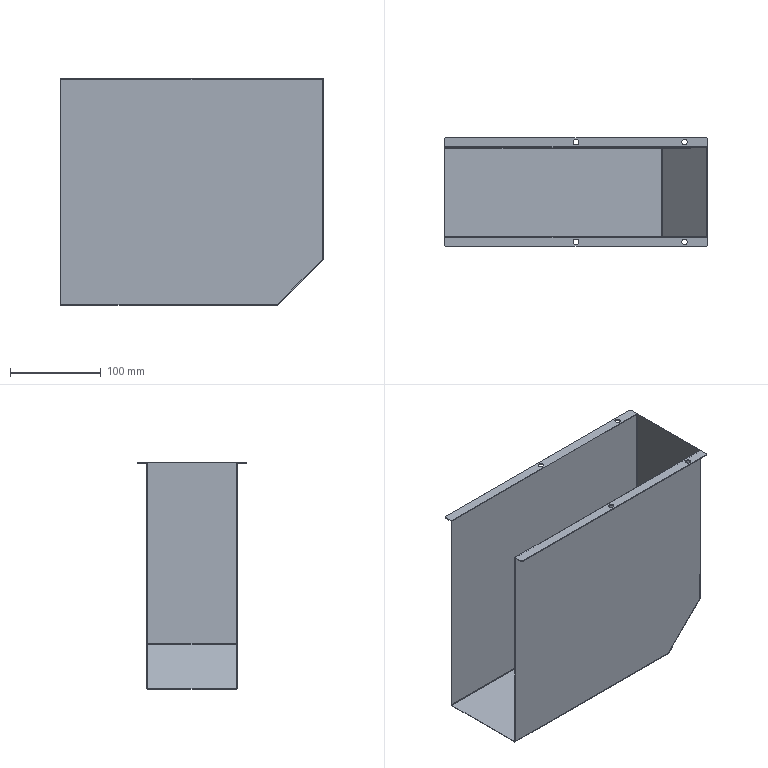Part | NX | features BREP 1 | 1 solid | 54 faces | box 290 x 120 x 250 mm | volume 102028 mm3 | cylinder 28 | plane 18 | sphere 8 | commonest cylinder face diameters 2 x12 1 x8 6 x8
STEP:
#1=CARTESIAN_POINT('',(-3.,55.,250.));
#2=VERTEX_POINT('',#1);
#3=CARTESIAN_POINT('',(3.,55.,250.));
#4=VERTEX_POINT('',#3);
#5=CARTESIAN_POINT('',(0.,55.,250.));
#6=DIRECTION('',(0.,0.,1.));
#7=DIRECTION('',(-1.,0.,0.));
#8=AXIS2_PLACEMENT_3D('',#5,#6,#7);
#9=CIRCLE('',#8,3.);
#10=EDGE_CURVE('',#2,#4,#9,.T.);
#11=ORIENTED_EDGE('',*,*,#10,.T.);
#12=CARTESIAN_POINT('',(3.,55.,249.));
#13=VERTEX_POINT('',#12);
#14=CARTESIAN_POINT('',(3.,55.,250.));
#15=DIRECTION('',(0.,0.,-1.));
#16=VECTOR('',#15,1000.);
#17=LINE('',#14,#16);
#18=EDGE_CURVE('',#4,#13,#17,.T.);
#19=ORIENTED_EDGE('',*,*,#18,.T.);
#20=CARTESIAN_POINT('',(-3.,55.,249.));
#21=VERTEX_POINT('',#20);
#22=CARTESIAN_POINT('',(0.,55.,249.));
#23=DIRECTION('',(0.,0.,1.));
#24=DIRECTION('',(-1.,0.,0.));
#25=AXIS2_PLACEMENT_3D('',#22,#23,#24);
#26=CIRCLE('',#25,3.);
#27=EDGE_CURVE('',#21,#13,#26,.T.);
#28=ORIENTED_EDGE('',*,*,#27,.F.);
#29=CARTESIAN_POINT('',(-3.,55.,250.));
#30=DIRECTION('',(0.,0.,-1.));
#31=VECTOR('',#30,1000.);
#32=LINE('',#29,#31);
#33=EDGE_CURVE('',#2,#21,#32,.T.);
#34=ORIENTED_EDGE('',*,*,#33,.F.);
#35=EDGE_LOOP('',(#11,#19,#28,#34));
#36=FACE_BOUND('',#35,.T.);
#37=CARTESIAN_POINT('',(0.,55.,250.));
#38=DIRECTION('',(0.,0.,-1.));
#39=DIRECTION('',(-1.,0.,0.));
#40=AXIS2_PLACEMENT_3D('',#37,#38,#39);
#41=CYLINDRICAL_SURFACE('',#40,3.);
#42=ADVANCED_FACE('',(#36),#41,.F.);
#43=CARTESIAN_POINT('',(117.,55.,250.));
#44=VERTEX_POINT('',#43);
#45=CARTESIAN_POINT('',(123.,55.,250.));
#46=VERTEX_POINT('',#45);
#47=CARTESIAN_POINT('',(120.,55.,250.));
#48=DIRECTION('',(0.,0.,1.));
#49=DIRECTION('',(-1.,0.,0.));
#50=AXIS2_PLACEMENT_3D('',#47,#48,#49);
#51=CIRCLE('',#50,3.);
#52=EDGE_CURVE('',#44,#46,#51,.T.);
#53=ORIENTED_EDGE('',*,*,#52,.T.);
#54=CARTESIAN_POINT('',(123.,55.,249.));
#55=VERTEX_POINT('',#54);
#56=CARTESIAN_POINT('',(123.,55.,250.));
#57=DIRECTION('',(0.,0.,-1.));
#58=VECTOR('',#57,1000.);
#59=LINE('',#56,#58);
#60=EDGE_CURVE('',#46,#55,#59,.T.);
#61=ORIENTED_EDGE('',*,*,#60,.T.);
#62=CARTESIAN_POINT('',(117.,55.,249.));
#63=VERTEX_POINT('',#62);
#64=CARTESIAN_POINT('',(120.,55.,249.));
#65=DIRECTION('',(0.,0.,1.));
#66=DIRECTION('',(-1.,0.,0.));
#67=AXIS2_PLACEMENT_3D('',#64,#65,#66);
#68=CIRCLE('',#67,3.);
#69=EDGE_CURVE('',#63,#55,#68,.T.);
#70=ORIENTED_EDGE('',*,*,#69,.F.);
#71=CARTESIAN_POINT('',(117.,55.,250.));
#72=DIRECTION('',(0.,0.,-1.));
#73=VECTOR('',#72,1000.);
#74=LINE('',#71,#73);
#75=EDGE_CURVE('',#44,#63,#74,.T.);
#76=ORIENTED_EDGE('',*,*,#75,.F.);
#77=EDGE_LOOP('',(#53,#61,#70,#76));
#78=FACE_BOUND('',#77,.T.);
#79=CARTESIAN_POINT('',(120.,55.,250.));
#80=DIRECTION('',(0.,0.,-1.));
#81=DIRECTION('',(-1.,0.,0.));
#82=AXIS2_PLACEMENT_3D('',#79,#80,#81);
#83=CYLINDRICAL_SURFACE('',#82,3.);
#84=ADVANCED_FACE('',(#78),#83,.F.);
#85=CARTESIAN_POINT('',(3.,-55.,250.));
#86=VERTEX_POINT('',#85);
#87=CARTESIAN_POINT('',(-3.,-55.,250.));
#88=VERTEX_POINT('',#87);
#89=CARTESIAN_POINT('',(0.,-55.,250.));
#90=DIRECTION('',(0.,0.,-1.));
#91=DIRECTION('',(-1.,0.,0.));
#92=AXIS2_PLACEMENT_3D('',#89,#90,#91);
#93=CIRCLE('',#92,3.);
#94=EDGE_CURVE('',#86,#88,#93,.T.);
#95=ORIENTED_EDGE('',*,*,#94,.F.);
#96=CARTESIAN_POINT('',(3.,-55.,249.));
#97=VERTEX_POINT('',#96);
#98=CARTESIAN_POINT('',(3.,-55.,250.));
#99=DIRECTION('',(0.,0.,-1.));
#100=VECTOR('',#99,1000.);
#101=LINE('',#98,#100);
#102=EDGE_CURVE('',#86,#97,#101,.T.);
#103=ORIENTED_EDGE('',*,*,#102,.T.);
#104=CARTESIAN_POINT('',(-3.,-55.,249.));
#105=VERTEX_POINT('',#104);
#106=CARTESIAN_POINT('',(0.,-55.,249.));
#107=DIRECTION('',(0.,0.,-1.));
#108=DIRECTION('',(-1.,0.,0.));
#109=AXIS2_PLACEMENT_3D('',#106,#107,#108);
#110=CIRCLE('',#109,3.);
#111=EDGE_CURVE('',#97,#105,#110,.T.);
#112=ORIENTED_EDGE('',*,*,#111,.T.);
#113=CARTESIAN_POINT('',(-3.,-55.,250.));
#114=DIRECTION('',(0.,0.,-1.));
#115=VECTOR('',#114,1000.);
#116=LINE('',#113,#115);
#117=EDGE_CURVE('',#88,#105,#116,.T.);
#118=ORIENTED_EDGE('',*,*,#117,.F.);
#119=EDGE_LOOP('',(#95,#103,#112,#118));
#120=FACE_BOUND('',#119,.T.);
#121=CARTESIAN_POINT('',(0.,-55.,250.));
#122=DIRECTION('',(0.,0.,-1.));
#123=DIRECTION('',(-1.,0.,0.));
#124=AXIS2_PLACEMENT_3D('',#121,#122,#123);
#125=CYLINDRICAL_SURFACE('',#124,3.);
#126=ADVANCED_FACE('',(#120),#125,.F.);
#127=CARTESIAN_POINT('',(123.,-55.,250.));
#128=VERTEX_POINT('',#127);
#129=CARTESIAN_POINT('',(117.,-55.,250.));
#130=VERTEX_POINT('',#129);
#131=CARTESIAN_POINT('',(120.,-55.,250.));
#132=DIRECTION('',(0.,0.,-1.));
#133=DIRECTION('',(-1.,0.,0.));
#134=AXIS2_PLACEMENT_3D('',#131,#132,#133);
#135=CIRCLE('',#134,3.);
#136=EDGE_CURVE('',#128,#130,#135,.T.);
#137=ORIENTED_EDGE('',*,*,#136,.F.);
#138=CARTESIAN_POINT('',(123.,-55.,249.));
#139=VERTEX_POINT('',#138);
#140=CARTESIAN_POINT('',(123.,-55.,250.));
#141=DIRECTION('',(0.,0.,-1.));
#142=VECTOR('',#141,1000.);
#143=LINE('',#140,#142);
#144=EDGE_CURVE('',#128,#139,#143,.T.);
#145=ORIENTED_EDGE('',*,*,#144,.T.);
#146=CARTESIAN_POINT('',(117.,-55.,249.));
#147=VERTEX_POINT('',#146);
#148=CARTESIAN_POINT('',(120.,-55.,249.));
#149=DIRECTION('',(0.,0.,-1.));
#150=DIRECTION('',(-1.,0.,0.));
#151=AXIS2_PLACEMENT_3D('',#148,#149,#150);
#152=CIRCLE('',#151,3.);
#153=EDGE_CURVE('',#139,#147,#152,.T.);
#154=ORIENTED_EDGE('',*,*,#153,.T.);
#155=CARTESIAN_POINT('',(117.,-55.,250.));
#156=DIRECTION('',(0.,0.,-1.));
#157=VECTOR('',#156,1000.);
#158=LINE('',#155,#157);
#159=EDGE_CURVE('',#130,#147,#158,.T.);
#160=ORIENTED_EDGE('',*,*,#159,.F.);
#161=EDGE_LOOP('',(#137,#145,#154,#160));
#162=FACE_BOUND('',#161,.T.);
#163=CARTESIAN_POINT('',(120.,-55.,250.));
#164=DIRECTION('',(0.,0.,-1.));
#165=DIRECTION('',(-1.,0.,0.));
#166=AXIS2_PLACEMENT_3D('',#163,#164,#165);
#167=CYLINDRICAL_SURFACE('',#166,3.);
#168=ADVANCED_FACE('',(#162),#167,.F.);
#169=CARTESIAN_POINT('',(144.,60.,250.));
#170=VERTEX_POINT('',#169);
#171=CARTESIAN_POINT('',(-144.,60.,250.));
#172=VERTEX_POINT('',#171);
#173=CARTESIAN_POINT('',(145.,60.,250.));
#174=DIRECTION('',(-1.,0.,0.));
#175=VECTOR('',#174,1000.);
#176=LINE('',#173,#175);
#177=EDGE_CURVE('',#170,#172,#176,.T.);
#178=ORIENTED_EDGE('',*,*,#177,.T.);
#179=CARTESIAN_POINT('',(-145.,59.,250.));
#180=VERTEX_POINT('',#179);
#181=CARTESIAN_POINT('',(-144.,59.,250.));
#182=DIRECTION('',(0.,0.,1.));
#183=DIRECTION('',(-1.,0.,0.));
#184=AXIS2_PLACEMENT_3D('',#181,#182,#183);
#185=CIRCLE('',#184,1.);
#186=EDGE_CURVE('',#172,#180,#185,.T.);
#187=ORIENTED_EDGE('',*,*,#186,.T.);
#188=CARTESIAN_POINT('',(-145.,49.5,250.));
#189=VERTEX_POINT('',#188);
#190=CARTESIAN_POINT('',(-145.,-50.,250.));
#191=DIRECTION('',(0.,-1.,0.));
#192=VECTOR('',#191,1000.);
#193=LINE('',#190,#192);
#194=EDGE_CURVE('',#180,#189,#193,.T.);
#195=ORIENTED_EDGE('',*,*,#194,.T.);
#196=CARTESIAN_POINT('',(144.,49.5,250.));
#197=VERTEX_POINT('',#196);
#198=CARTESIAN_POINT('',(0.,49.5,250.));
#199=DIRECTION('',(-1.,0.,0.));
#200=VECTOR('',#199,1000.);
#201=LINE('',#198,#200);
#202=EDGE_CURVE('',#197,#189,#201,.T.);
#203=ORIENTED_EDGE('',*,*,#202,.F.);
#204=CARTESIAN_POINT('',(144.5,49.,250.));
#205=VERTEX_POINT('',#204);
#206=CARTESIAN_POINT('',(144.,49.,250.));
#207=DIRECTION('',(0.,0.,-1.));
#208=DIRECTION('',(-1.,0.,0.));
#209=AXIS2_PLACEMENT_3D('',#206,#207,#208);
#210=CIRCLE('',#209,0.5);
#211=EDGE_CURVE('',#197,#205,#210,.T.);
#212=ORIENTED_EDGE('',*,*,#211,.T.);
#213=CARTESIAN_POINT('',(144.5,-49.,250.));
#214=VERTEX_POINT('',#213);
#215=CARTESIAN_POINT('',(144.5,0.,250.));
#216=DIRECTION('',(0.,1.,0.));
#217=VECTOR('',#216,1000.);
#218=LINE('',#215,#217);
#219=EDGE_CURVE('',#214,#205,#218,.T.);
#220=ORIENTED_EDGE('',*,*,#219,.F.);
#221=CARTESIAN_POINT('',(144.,-49.5,250.));
#222=VERTEX_POINT('',#221);
#223=CARTESIAN_POINT('',(144.,-49.,250.));
#224=DIRECTION('',(0.,0.,-1.));
#225=DIRECTION('',(-1.,0.,0.));
#226=AXIS2_PLACEMENT_3D('',#223,#224,#225);
#227=CIRCLE('',#226,0.5);
#228=EDGE_CURVE('',#214,#222,#227,.T.);
#229=ORIENTED_EDGE('',*,*,#228,.T.);
#230=CARTESIAN_POINT('',(-145.,-49.5,250.));
#231=VERTEX_POINT('',#230);
#232=CARTESIAN_POINT('',(0.,-49.5,250.));
#233=DIRECTION('',(1.,0.,0.));
#234=VECTOR('',#233,1000.);
#235=LINE('',#232,#234);
#236=EDGE_CURVE('',#231,#222,#235,.T.);
#237=ORIENTED_EDGE('',*,*,#236,.F.);
#238=CARTESIAN_POINT('',(-145.,-59.,250.));
#239=VERTEX_POINT('',#238);
#240=CARTESIAN_POINT('',(-145.,-50.,250.));
#241=DIRECTION('',(0.,-1.,0.));
#242=VECTOR('',#241,1000.);
#243=LINE('',#240,#242);
#244=EDGE_CURVE('',#231,#239,#243,.T.);
#245=ORIENTED_EDGE('',*,*,#244,.T.);
#246=CARTESIAN_POINT('',(-144.,-60.,250.));
#247=VERTEX_POINT('',#246);
#248=CARTESIAN_POINT('',(-144.,-59.,250.));
#249=DIRECTION('',(0.,0.,1.));
#250=DIRECTION('',(-1.,0.,0.));
#251=AXIS2_PLACEMENT_3D('',#248,#249,#250);
#252=CIRCLE('',#251,1.);
#253=EDGE_CURVE('',#239,#247,#252,.T.);
#254=ORIENTED_EDGE('',*,*,#253,.T.);
#255=CARTESIAN_POINT('',(144.,-60.,250.));
#256=VERTEX_POINT('',#255);
#257=CARTESIAN_POINT('',(145.,-60.,250.));
#258=DIRECTION('',(-1.,0.,0.));
#259=VECTOR('',#258,1000.);
#260=LINE('',#257,#259);
#261=EDGE_CURVE('',#256,#247,#260,.T.);
#262=ORIENTED_EDGE('',*,*,#261,.F.);
#263=CARTESIAN_POINT('',(145.,-59.,250.));
#264=VERTEX_POINT('',#263);
#265=CARTESIAN_POINT('',(144.,-59.,250.));
#266=DIRECTION('',(0.,0.,1.));
#267=DIRECTION('',(-1.,0.,0.));
#268=AXIS2_PLACEMENT_3D('',#265,#266,#267);
#269=CIRCLE('',#268,1.);
#270=EDGE_CURVE('',#256,#264,#269,.T.);
#271=ORIENTED_EDGE('',*,*,#270,.T.);
#272=CARTESIAN_POINT('',(145.,49.,250.));
#273=VERTEX_POINT('',#272);
#274=CARTESIAN_POINT('',(145.,-50.,250.));
#275=DIRECTION('',(0.,1.,0.));
#276=VECTOR('',#275,1000.);
#277=LINE('',#274,#276);
#278=EDGE_CURVE('',#264,#273,#277,.T.);
#279=ORIENTED_EDGE('',*,*,#278,.T.);
#280=CARTESIAN_POINT('',(144.,50.,250.));
#281=VERTEX_POINT('',#280);
#282=CARTESIAN_POINT('',(144.,49.,250.));
#283=DIRECTION('',(0.,0.,1.));
#284=DIRECTION('',(-1.,0.,0.));
#285=AXIS2_PLACEMENT_3D('',#282,#283,#284);
#286=CIRCLE('',#285,1.);
#287=EDGE_CURVE('',#273,#281,#286,.T.);
#288=ORIENTED_EDGE('',*,*,#287,.T.);
#289=CARTESIAN_POINT('',(145.,50.,250.));
#290=VERTEX_POINT('',#289);
#291=CARTESIAN_POINT('',(145.,50.,250.));
#292=DIRECTION('',(-1.,0.,0.));
#293=VECTOR('',#292,1000.);
#294=LINE('',#291,#293);
#295=EDGE_CURVE('',#290,#281,#294,.T.);
#296=ORIENTED_EDGE('',*,*,#295,.F.);
#297=CARTESIAN_POINT('',(145.,59.,250.));
#298=VERTEX_POINT('',#297);
#299=CARTESIAN_POINT('',(145.,60.,250.));
#300=DIRECTION('',(0.,-1.,0.));
#301=VECTOR('',#300,1000.);
#302=LINE('',#299,#301);
#303=EDGE_CURVE('',#298,#290,#302,.T.);
#304=ORIENTED_EDGE('',*,*,#303,.F.);
#305=CARTESIAN_POINT('',(144.,59.,250.));
#306=DIRECTION('',(0.,0.,1.));
#307=DIRECTION('',(-1.,0.,0.));
#308=AXIS2_PLACEMENT_3D('',#305,#306,#307);
#309=CIRCLE('',#308,1.);
#310=EDGE_CURVE('',#298,#170,#309,.T.);
#311=ORIENTED_EDGE('',*,*,#310,.T.);
#312=EDGE_LOOP('',(#178,#187,#195,#203,#212,#220,#229,#237,#245,#254,#262,#271,#279,#288,#296,#304,#311));
#313=FACE_BOUND('',#312,.T.);
#314=ORIENTED_EDGE('',*,*,#52,.F.);
#315=CARTESIAN_POINT('',(120.,55.,250.));
#316=DIRECTION('',(0.,0.,1.));
#317=DIRECTION('',(-1.,0.,0.));
#318=AXIS2_PLACEMENT_3D('',#315,#316,#317);
#319=CIRCLE('',#318,3.);
#320=EDGE_CURVE('',#46,#44,#319,.T.);
#321=ORIENTED_EDGE('',*,*,#320,.F.);
#322=EDGE_LOOP('',(#314,#321));
#323=FACE_BOUND('',#322,.T.);
#324=CARTESIAN_POINT('',(0.,-55.,250.));
#325=DIRECTION('',(0.,0.,-1.));
#326=DIRECTION('',(-1.,0.,0.));
#327=AXIS2_PLACEMENT_3D('',#324,#325,#326);
#328=CIRCLE('',#327,3.);
#329=EDGE_CURVE('',#88,#86,#328,.T.);
#330=ORIENTED_EDGE('',*,*,#329,.T.);
#331=ORIENTED_EDGE('',*,*,#94,.T.);
#332=EDGE_LOOP('',(#330,#331));
#333=FACE_BOUND('',#332,.T.);
#334=CARTESIAN_POINT('',(120.,-55.,250.));
#335=DIRECTION('',(0.,0.,-1.));
#336=DIRECTION('',(-1.,0.,0.));
#337=AXIS2_PLACEMENT_3D('',#334,#335,#336);
#338=CIRCLE('',#337,3.);
#339=EDGE_CURVE('',#130,#128,#338,.T.);
#340=ORIENTED_EDGE('',*,*,#339,.T.);
#341=ORIENTED_EDGE('',*,*,#136,.T.);
#342=EDGE_LOOP('',(#340,#341));
#343=FACE_BOUND('',#342,.T.);
#344=ORIENTED_EDGE('',*,*,#10,.F.);
#345=CARTESIAN_POINT('',(0.,55.,250.));
#346=DIRECTION('',(0.,0.,1.));
#347=DIRECTION('',(-1.,0.,0.));
#348=AXIS2_PLACEMENT_3D('',#345,#346,#347);
#349=CIRCLE('',#348,3.);
#350=EDGE_CURVE('',#4,#2,#349,.T.);
#351=ORIENTED_EDGE('',*,*,#350,.F.);
#352=EDGE_LOOP('',(#344,#351));
#353=FACE_BOUND('',#352,.T.);
#354=CARTESIAN_POINT('',(0.,0.,250.));
#355=DIRECTION('',(0.,0.,-1.));
#356=DIRECTION('',(0.,-1.,0.));
#357=AXIS2_PLACEMENT_3D('',#354,#355,#356);
#358=PLANE('',#357);
#359=ADVANCED_FACE('',(#313,#323,#333,#343,#353),#358,.F.);
#360=CARTESIAN_POINT('',(-145.,59.,249.));
#361=VERTEX_POINT('',#360);
#362=CARTESIAN_POINT('',(-145.,50.,249.));
#363=VERTEX_POINT('',#362);
#364=CARTESIAN_POINT('',(-145.,60.,249.));
#365=DIRECTION('',(0.,-1.,0.));
#366=VECTOR('',#365,1000.);
#367=LINE('',#364,#366);
#368=EDGE_CURVE('',#361,#363,#367,.T.);
#369=ORIENTED_EDGE('',*,*,#368,.F.);
#370=CARTESIAN_POINT('',(-144.,60.,249.));
#371=VERTEX_POINT('',#370);
#372=CARTESIAN_POINT('',(-144.,59.,249.));
#373=DIRECTION('',(0.,0.,-1.));
#374=DIRECTION('',(-1.,0.,0.));
#375=AXIS2_PLACEMENT_3D('',#372,#373,#374);
#376=CIRCLE('',#375,1.);
#377=EDGE_CURVE('',#361,#371,#376,.T.);
#378=ORIENTED_EDGE('',*,*,#377,.T.);
#379=CARTESIAN_POINT('',(144.,60.,249.));
#380=VERTEX_POINT('',#379);
#381=CARTESIAN_POINT('',(145.,60.,249.));
#382=DIRECTION('',(1.,0.,0.));
#383=VECTOR('',#382,1000.);
#384=LINE('',#381,#383);
#385=EDGE_CURVE('',#371,#380,#384,.T.);
#386=ORIENTED_EDGE('',*,*,#385,.T.);
#387=CARTESIAN_POINT('',(145.,59.,249.));
#388=VERTEX_POINT('',#387);
#389=CARTESIAN_POINT('',(144.,59.,249.));
#390=DIRECTION('',(0.,0.,-1.));
#391=DIRECTION('',(-1.,0.,0.));
#392=AXIS2_PLACEMENT_3D('',#389,#390,#391);
#393=CIRCLE('',#392,1.);
#394=EDGE_CURVE('',#380,#388,#393,.T.);
#395=ORIENTED_EDGE('',*,*,#394,.T.);
#396=CARTESIAN_POINT('',(145.,50.,249.));
#397=VERTEX_POINT('',#396);
#398=CARTESIAN_POINT('',(145.,60.,249.));
#399=DIRECTION('',(0.,-1.,0.));
#400=VECTOR('',#399,1000.);
#401=LINE('',#398,#400);
#402=EDGE_CURVE('',#388,#397,#401,.T.);
#403=ORIENTED_EDGE('',*,*,#402,.T.);
#404=CARTESIAN_POINT('',(144.,50.,249.));
#405=VERTEX_POINT('',#404);
#406=CARTESIAN_POINT('',(145.,50.,249.));
#407=DIRECTION('',(1.,0.,0.));
#408=VECTOR('',#407,1000.);
#409=LINE('',#406,#408);
#410=EDGE_CURVE('',#405,#397,#409,.T.);
#411=ORIENTED_EDGE('',*,*,#410,.F.);
#412=CARTESIAN_POINT('',(145.,50.,249.));
#413=DIRECTION('',(1.,0.,0.));
#414=VECTOR('',#413,1000.);
#415=LINE('',#412,#414);
#416=EDGE_CURVE('',#363,#405,#415,.T.);
#417=ORIENTED_EDGE('',*,*,#416,.F.);
#418=EDGE_LOOP('',(#369,#378,#386,#395,#403,#411,#417));
#419=FACE_BOUND('',#418,.T.);
#420=ORIENTED_EDGE('',*,*,#69,.T.);
#421=CARTESIAN_POINT('',(120.,55.,249.));
#422=DIRECTION('',(0.,0.,1.));
#423=DIRECTION('',(-1.,0.,0.));
#424=AXIS2_PLACEMENT_3D('',#421,#422,#423);
#425=CIRCLE('',#424,3.);
#426=EDGE_CURVE('',#55,#63,#425,.T.);
#427=ORIENTED_EDGE('',*,*,#426,.T.);
#428=EDGE_LOOP('',(#420,#427));
#429=FACE_BOUND('',#428,.T.);
#430=ORIENTED_EDGE('',*,*,#27,.T.);
#431=CARTESIAN_POINT('',(0.,55.,249.));
#432=DIRECTION('',(0.,0.,1.));
#433=DIRECTION('',(-1.,0.,0.));
#434=AXIS2_PLACEMENT_3D('',#431,#432,#433);
#435=CIRCLE('',#434,3.);
#436=EDGE_CURVE('',#13,#21,#435,.T.);
#437=ORIENTED_EDGE('',*,*,#436,.T.);
#438=EDGE_LOOP('',(#430,#437));
#439=FACE_BOUND('',#438,.T.);
#440=CARTESIAN_POINT('',(145.,60.,249.));
#441=DIRECTION('',(0.,0.,-1.));
#442=DIRECTION('',(0.,-1.,0.));
#443=AXIS2_PLACEMENT_3D('',#440,#441,#442);
#444=PLANE('',#443);
#445=ADVANCED_FACE('',(#419,#429,#439),#444,.T.);
#446=CARTESIAN_POINT('',(94.586,-50.,1.));
#447=VERTEX_POINT('',#446);
#448=CARTESIAN_POINT('',(144.,-50.,50.414));
#449=VERTEX_POINT('',#448);
#450=CARTESIAN_POINT('',(144.293,-50.,50.707));
#451=DIRECTION('',(0.7071,0.,0.7071));
#452=VECTOR('',#451,1000.);
#453=LINE('',#450,#452);
#454=EDGE_CURVE('',#447,#449,#453,.T.);
#455=ORIENTED_EDGE('',*,*,#454,.T.);
#456=CARTESIAN_POINT('',(144.,-50.,249.));
#457=VERTEX_POINT('',#456);
#458=CARTESIAN_POINT('',(144.,-50.,250.));
#459=DIRECTION('',(0.,0.,1.));
#460=VECTOR('',#459,1000.);
#461=LINE('',#458,#460);
#462=EDGE_CURVE('',#449,#457,#461,.T.);
#463=ORIENTED_EDGE('',*,*,#462,.T.);
#464=CARTESIAN_POINT('',(-145.,-50.,249.));
#465=VERTEX_POINT('',#464);
#466=CARTESIAN_POINT('',(145.,-50.,249.));
#467=DIRECTION('',(1.,0.,0.));
#468=VECTOR('',#467,1000.);
#469=LINE('',#466,#468);
#470=EDGE_CURVE('',#465,#457,#469,.T.);
#471=ORIENTED_EDGE('',*,*,#470,.F.);
#472=CARTESIAN_POINT('',(-145.,-50.,1.));
#473=VERTEX_POINT('',#472);
#474=CARTESIAN_POINT('',(-145.,-50.,250.));
#475=DIRECTION('',(0.,0.,-1.));
#476=VECTOR('',#475,1000.);
#477=LINE('',#474,#476);
#478=EDGE_CURVE('',#465,#473,#477,.T.);
#479=ORIENTED_EDGE('',*,*,#478,.T.);
#480=CARTESIAN_POINT('',(95.,-50.,1.));
#481=DIRECTION('',(1.,0.,0.));
#482=VECTOR('',#481,1000.);
#483=LINE('',#480,#482);
#484=EDGE_CURVE('',#473,#447,#483,.T.);
#485=ORIENTED_EDGE('',*,*,#484,.T.);
#486=EDGE_LOOP('',(#455,#463,#471,#479,#485));
#487=FACE_BOUND('',#486,.T.);
#488=CARTESIAN_POINT('',(-145.,-50.,250.));
#489=DIRECTION('',(0.,1.,0.));
#490=DIRECTION('',(1.,0.,0.));
#491=AXIS2_PLACEMENT_3D('',#488,#489,#490);
#492=PLANE('',#491);
#493=ADVANCED_FACE('',(#487),#492,.F.);
#494=ORIENTED_EDGE('',*,*,#278,.F.);
#495=CARTESIAN_POINT('',(145.,-59.,249.));
#496=VERTEX_POINT('',#495);
#497=CARTESIAN_POINT('',(145.,-59.,250.));
#498=DIRECTION('',(0.,0.,-1.));
#499=VECTOR('',#498,1000.);
#500=LINE('',#497,#499);
#501=EDGE_CURVE('',#264,#496,#500,.T.);
#502=ORIENTED_EDGE('',*,*,#501,.T.);
#503=CARTESIAN_POINT('',(145.,-49.,249.));
#504=VERTEX_POINT('',#503);
#505=CARTESIAN_POINT('',(145.,-60.,249.));
#506=DIRECTION('',(0.,1.,0.));
#507=VECTOR('',#506,1000.);
#508=LINE('',#505,#507);
#509=EDGE_CURVE('',#496,#504,#508,.T.);
#510=ORIENTED_EDGE('',*,*,#509,.T.);
#511=CARTESIAN_POINT('',(145.,-49.,50.414));
#512=VERTEX_POINT('',#511);
#513=CARTESIAN_POINT('',(145.,-49.,250.));
#514=DIRECTION('',(0.,0.,-1.));
#515=VECTOR('',#514,1000.);
#516=LINE('',#513,#515);
#517=EDGE_CURVE('',#504,#512,#516,.T.);
#518=ORIENTED_EDGE('',*,*,#517,.T.);
#519=CARTESIAN_POINT('',(145.,49.,50.414));
#520=VERTEX_POINT('',#519);
#521=CARTESIAN_POINT('',(145.,50.,50.414));
#522=DIRECTION('',(0.,1.,0.));
#523=VECTOR('',#522,1000.);
#524=LINE('',#521,#523);
#525=EDGE_CURVE('',#512,#520,#524,.T.);
#526=ORIENTED_EDGE('',*,*,#525,.T.);
#527=CARTESIAN_POINT('',(145.,49.,250.));
#528=DIRECTION('',(0.,0.,1.));
#529=VECTOR('',#528,1000.);
#530=LINE('',#527,#529);
#531=EDGE_CURVE('',#520,#273,#530,.T.);
#532=ORIENTED_EDGE('',*,*,#531,.T.);
#533=EDGE_LOOP('',(#494,#502,#510,#518,#526,#532));
#534=FACE_BOUND('',#533,.T.);
#535=CARTESIAN_POINT('',(145.,-50.,250.));
#536=DIRECTION('',(-1.,0.,0.));
#537=DIRECTION('',(0.,0.,1.));
#538=AXIS2_PLACEMENT_3D('',#535,#536,#537);
#539=PLANE('',#538);
#540=ADVANCED_FACE('',(#534),#539,.F.);
#541=CARTESIAN_POINT('',(-145.,50.,1.));
#542=VERTEX_POINT('',#541);
#543=CARTESIAN_POINT('',(-145.,50.,250.));
#544=DIRECTION('',(0.,0.,-1.));
#545=VECTOR('',#544,1000.);
#546=LINE('',#543,#545);
#547=EDGE_CURVE('',#363,#542,#546,.T.);
#548=ORIENTED_EDGE('',*,*,#547,.F.);
#549=ORIENTED_EDGE('',*,*,#416,.T.);
#550=CARTESIAN_POINT('',(144.,50.,50.414));
#551=VERTEX_POINT('',#550);
#552=CARTESIAN_POINT('',(144.,50.,250.));
#553=DIRECTION('',(0.,0.,-1.));
#554=VECTOR('',#553,1000.);
#555=LINE('',#552,#554);
#556=EDGE_CURVE('',#405,#551,#555,.T.);
#557=ORIENTED_EDGE('',*,*,#556,.T.);
#558=CARTESIAN_POINT('',(94.586,50.,1.));
#559=VERTEX_POINT('',#558);
#560=CARTESIAN_POINT('',(94.293,50.,0.7071));
#561=DIRECTION('',(-0.7071,0.,-0.7071));
#562=VECTOR('',#561,1000.);
#563=LINE('',#560,#562);
#564=EDGE_CURVE('',#551,#559,#563,.T.);
#565=ORIENTED_EDGE('',*,*,#564,.T.);
#566=CARTESIAN_POINT('',(-145.,50.,1.));
#567=DIRECTION('',(-1.,0.,0.));
#568=VECTOR('',#567,1000.);
#569=LINE('',#566,#568);
#570=EDGE_CURVE('',#559,#542,#569,.T.);
#571=ORIENTED_EDGE('',*,*,#570,.T.);
#572=EDGE_LOOP('',(#548,#549,#557,#565,#571));
#573=FACE_BOUND('',#572,.T.);
#574=CARTESIAN_POINT('',(-145.,50.,250.));
#575=DIRECTION('',(0.,-1.,0.));
#576=DIRECTION('',(0.,0.,-1.));
#577=AXIS2_PLACEMENT_3D('',#574,#575,#576);
#578=PLANE('',#577);
#579=ADVANCED_FACE('',(#573),#578,.F.);
#580=ORIENTED_EDGE('',*,*,#194,.F.);
#581=CARTESIAN_POINT('',(-145.,59.,250.));
#582=DIRECTION('',(0.,0.,-1.));
#583=VECTOR('',#582,1000.);
#584=LINE('',#581,#583);
#585=EDGE_CURVE('',#180,#361,#584,.T.);
#586=ORIENTED_EDGE('',*,*,#585,.T.);
#587=ORIENTED_EDGE('',*,*,#368,.T.);
#588=ORIENTED_EDGE('',*,*,#547,.T.);
#589=CARTESIAN_POINT('',(-145.,49.,0.));
#590=VERTEX_POINT('',#589);
#591=CARTESIAN_POINT('',(-145.,49.,1.));
#592=DIRECTION('',(-1.,0.,0.));
#593=DIRECTION('',(0.,0.,-1.));
#594=AXIS2_PLACEMENT_3D('',#591,#592,#593);
#595=CIRCLE('',#594,1.);
#596=EDGE_CURVE('',#542,#590,#595,.T.);
#597=ORIENTED_EDGE('',*,*,#596,.T.);
#598=CARTESIAN_POINT('',(-145.,-49.,0.));
#599=VERTEX_POINT('',#598);
#600=CARTESIAN_POINT('',(-145.,-50.,0.));
#601=DIRECTION('',(0.,-1.,0.));
#602=VECTOR('',#601,1000.);
#603=LINE('',#600,#602);
#604=EDGE_CURVE('',#590,#599,#603,.T.);
#605=ORIENTED_EDGE('',*,*,#604,.T.);
#606=CARTESIAN_POINT('',(-145.,-49.,1.));
#607=DIRECTION('',(-1.,0.,0.));
#608=DIRECTION('',(0.,0.,-1.));
#609=AXIS2_PLACEMENT_3D('',#606,#607,#608);
#610=CIRCLE('',#609,1.);
#611=EDGE_CURVE('',#599,#473,#610,.T.);
#612=ORIENTED_EDGE('',*,*,#611,.T.);
#613=ORIENTED_EDGE('',*,*,#478,.F.);
#614=CARTESIAN_POINT('',(-145.,-59.,249.));
#615=VERTEX_POINT('',#614);
#616=CARTESIAN_POINT('',(-145.,-60.,249.));
#617=DIRECTION('',(0.,1.,0.));
#618=VECTOR('',#617,1000.);
#619=LINE('',#616,#618);
#620=EDGE_CURVE('',#615,#465,#619,.T.);
#621=ORIENTED_EDGE('',*,*,#620,.F.);
#622=CARTESIAN_POINT('',(-145.,-59.,250.));
#623=DIRECTION('',(0.,0.,1.));
#624=VECTOR('',#623,1000.);
#625=LINE('',#622,#624);
#626=EDGE_CURVE('',#615,#239,#625,.T.);
#627=ORIENTED_EDGE('',*,*,#626,.T.);
#628=ORIENTED_EDGE('',*,*,#244,.F.);
#629=CARTESIAN_POINT('',(-145.,-49.5,1.));
#630=VERTEX_POINT('',#629);
#631=CARTESIAN_POINT('',(-145.,-49.5,250.));
#632=DIRECTION('',(0.,0.,-1.));
#633=VECTOR('',#632,1000.);
#634=LINE('',#631,#633);
#635=EDGE_CURVE('',#231,#630,#634,.T.);
#636=ORIENTED_EDGE('',*,*,#635,.T.);
#637=CARTESIAN_POINT('',(-145.,-49.,0.5));
#638=VERTEX_POINT('',#637);
#639=CARTESIAN_POINT('',(-145.,-49.,1.));
#640=DIRECTION('',(1.,0.,0.));
#641=DIRECTION('',(0.,0.,-1.));
#642=AXIS2_PLACEMENT_3D('',#639,#640,#641);
#643=CIRCLE('',#642,0.5);
#644=EDGE_CURVE('',#630,#638,#643,.T.);
#645=ORIENTED_EDGE('',*,*,#644,.T.);
#646=CARTESIAN_POINT('',(-145.,49.,0.5));
#647=VERTEX_POINT('',#646);
#648=CARTESIAN_POINT('',(-145.,-49.5,0.5));
#649=DIRECTION('',(0.,1.,0.));
#650=VECTOR('',#649,1000.);
#651=LINE('',#648,#650);
#652=EDGE_CURVE('',#638,#647,#651,.T.);
#653=ORIENTED_EDGE('',*,*,#652,.T.);
#654=CARTESIAN_POINT('',(-145.,49.5,1.));
#655=VERTEX_POINT('',#654);
#656=CARTESIAN_POINT('',(-145.,49.,1.));
#657=DIRECTION('',(1.,0.,0.));
#658=DIRECTION('',(0.,0.,-1.));
#659=AXIS2_PLACEMENT_3D('',#656,#657,#658);
#660=CIRCLE('',#659,0.5);
#661=EDGE_CURVE('',#647,#655,#660,.T.);
#662=ORIENTED_EDGE('',*,*,#661,.T.);
#663=CARTESIAN_POINT('',(-145.,49.5,0.5));
#664=DIRECTION('',(0.,0.,1.));
#665=VECTOR('',#664,1000.);
#666=LINE('',#663,#665);
#667=EDGE_CURVE('',#655,#189,#666,.T.);
#668=ORIENTED_EDGE('',*,*,#667,.T.);
#669=EDGE_LOOP('',(#580,#586,#587,#588,#597,#605,#612,#613,#621,#627,#628,#636,#645,#653,#662,#668));
#670=FACE_BOUND('',#669,.T.);
#671=CARTESIAN_POINT('',(-145.,-50.,250.));
#672=DIRECTION('',(1.,0.,0.));
#673=DIRECTION('',(0.,1.,0.));
#674=AXIS2_PLACEMENT_3D('',#671,#672,#673);
#675=PLANE('',#674);
#676=ADVANCED_FACE('',(#670),#675,.F.);
#677=CARTESIAN_POINT('',(94.586,49.,0.));
#678=VERTEX_POINT('',#677);
#679=CARTESIAN_POINT('',(94.586,-49.,0.));
#680=VERTEX_POINT('',#679);
#681=CARTESIAN_POINT('',(94.586,0.,0.));
#682=DIRECTION('',(0.,-1.,0.));
#683=VECTOR('',#682,1000.);
#684=LINE('',#681,#683);
#685=EDGE_CURVE('',#678,#680,#684,.T.);
#686=ORIENTED_EDGE('',*,*,#685,.T.);
#687=CARTESIAN_POINT('',(-145.,-49.,0.));
#688=DIRECTION('',(-1.,0.,0.));
#689=VECTOR('',#688,1000.);
#690=LINE('',#687,#689);
#691=EDGE_CURVE('',#680,#599,#690,.T.);
#692=ORIENTED_EDGE('',*,*,#691,.T.);
#693=ORIENTED_EDGE('',*,*,#604,.F.);
#694=CARTESIAN_POINT('',(95.,49.,0.));
#695=DIRECTION('',(1.,0.,0.));
#696=VECTOR('',#695,1000.);
#697=LINE('',#694,#696);
#698=EDGE_CURVE('',#590,#678,#697,.T.);
#699=ORIENTED_EDGE('',*,*,#698,.T.);
#700=EDGE_LOOP('',(#686,#692,#693,#699));
#701=FACE_BOUND('',#700,.T.);
#702=CARTESIAN_POINT('',(0.,0.,0.));
#703=DIRECTION('',(0.,0.,-1.));
#704=DIRECTION('',(0.,-1.,0.));
#705=AXIS2_PLACEMENT_3D('',#702,#703,#704);
#706=PLANE('',#705);
#707=ADVANCED_FACE('',(#701),#706,.T.);
#708=CARTESIAN_POINT('',(144.707,49.,49.707));
#709=VERTEX_POINT('',#708);
#710=CARTESIAN_POINT('',(144.707,-49.,49.707));
#711=VERTEX_POINT('',#710);
#712=CARTESIAN_POINT('',(144.707,-50.,49.707));
#713=DIRECTION('',(0.,-1.,0.));
#714=VECTOR('',#713,1000.);
#715=LINE('',#712,#714);
#716=EDGE_CURVE('',#709,#711,#715,.T.);
#717=ORIENTED_EDGE('',*,*,#716,.T.);
#718=CARTESIAN_POINT('',(95.293,-49.,0.2929));
#719=VERTEX_POINT('',#718);
#720=CARTESIAN_POINT('',(95.,-49.,0.));
#721=DIRECTION('',(-0.7071,0.,-0.7071));
#722=VECTOR('',#721,1000.);
#723=LINE('',#720,#722);
#724=EDGE_CURVE('',#711,#719,#723,.T.);
#725=ORIENTED_EDGE('',*,*,#724,.T.);
#726=CARTESIAN_POINT('',(95.293,49.,0.2929));
#727=VERTEX_POINT('',#726);
#728=CARTESIAN_POINT('',(95.293,-50.,0.2929));
#729=DIRECTION('',(0.,1.,0.));
#730=VECTOR('',#729,1000.);
#731=LINE('',#728,#730);
#732=EDGE_CURVE('',#719,#727,#731,.T.);
#733=ORIENTED_EDGE('',*,*,#732,.T.);
#734=CARTESIAN_POINT('',(145.,49.,50.));
#735=DIRECTION('',(0.7071,0.,0.7071));
#736=VECTOR('',#735,1000.);
#737=LINE('',#734,#736);
#738=EDGE_CURVE('',#727,#709,#737,.T.);
#739=ORIENTED_EDGE('',*,*,#738,.T.);
#740=EDGE_LOOP('',(#717,#725,#733,#739));
#741=FACE_BOUND('',#740,.T.);
#742=CARTESIAN_POINT('',(145.,-50.,50.));
#743=DIRECTION('',(0.7071,0.,-0.7071));
#744=DIRECTION('',(0.,-1.,0.));
#745=AXIS2_PLACEMENT_3D('',#742,#743,#744);
#746=PLANE('',#745);
#747=ADVANCED_FACE('',(#741),#746,.T.);
#748=ORIENTED_EDGE('',*,*,#219,.T.);
#749=CARTESIAN_POINT('',(144.5,49.,50.414));
#750=VERTEX_POINT('',#749);
#751=CARTESIAN_POINT('',(144.5,49.,50.207));
#752=DIRECTION('',(0.,0.,-1.));
#753=VECTOR('',#752,1000.);
#754=LINE('',#751,#753);
#755=EDGE_CURVE('',#205,#750,#754,.T.);
#756=ORIENTED_EDGE('',*,*,#755,.T.);
#757=CARTESIAN_POINT('',(144.5,-49.,50.414));
#758=VERTEX_POINT('',#757);
#759=CARTESIAN_POINT('',(144.5,-50.,50.414));
#760=DIRECTION('',(0.,-1.,0.));
#761=VECTOR('',#760,1000.);
#762=LINE('',#759,#761);
#763=EDGE_CURVE('',#750,#758,#762,.T.);
#764=ORIENTED_EDGE('',*,*,#763,.T.);
#765=CARTESIAN_POINT('',(144.5,-49.,250.));
#766=DIRECTION('',(0.,0.,1.));
#767=VECTOR('',#766,1000.);
#768=LINE('',#765,#767);
#769=EDGE_CURVE('',#758,#214,#768,.T.);
#770=ORIENTED_EDGE('',*,*,#769,.T.);
#771=EDGE_LOOP('',(#748,#756,#764,#770));
#772=FACE_BOUND('',#771,.T.);
#773=CARTESIAN_POINT('',(144.5,-50.,250.));
#774=DIRECTION('',(-1.,0.,0.));
#775=DIRECTION('',(0.,0.,1.));
#776=AXIS2_PLACEMENT_3D('',#773,#774,#775);
#777=PLANE('',#776);
#778=ADVANCED_FACE('',(#772),#777,.T.);
#779=CARTESIAN_POINT('',(94.586,49.5,1.));
#780=VERTEX_POINT('',#779);
#781=CARTESIAN_POINT('',(144.,49.5,50.414));
#782=VERTEX_POINT('',#781);
#783=CARTESIAN_POINT('',(99.293,49.5,5.707));
#784=DIRECTION('',(0.7071,0.,0.7071));
#785=VECTOR('',#784,1000.);
#786=LINE('',#783,#785);
#787=EDGE_CURVE('',#780,#782,#786,.T.);
#788=ORIENTED_EDGE('',*,*,#787,.T.);
#789=CARTESIAN_POINT('',(144.,49.5,250.));
#790=DIRECTION('',(0.,0.,1.));
#791=VECTOR('',#790,1000.);
#792=LINE('',#789,#791);
#793=EDGE_CURVE('',#782,#197,#792,.T.);
#794=ORIENTED_EDGE('',*,*,#793,.T.);
#795=ORIENTED_EDGE('',*,*,#202,.T.);
#796=ORIENTED_EDGE('',*,*,#667,.F.);
#797=CARTESIAN_POINT('',(-145.,49.5,1.));
#798=DIRECTION('',(1.,0.,0.));
#799=VECTOR('',#798,1000.);
#800=LINE('',#797,#799);
#801=EDGE_CURVE('',#655,#780,#800,.T.);
#802=ORIENTED_EDGE('',*,*,#801,.T.);
#803=EDGE_LOOP('',(#788,#794,#795,#796,#802));
#804=FACE_BOUND('',#803,.T.);
#805=CARTESIAN_POINT('',(-145.,49.5,250.));
#806=DIRECTION('',(0.,-1.,0.));
#807=DIRECTION('',(0.,0.,-1.));
#808=AXIS2_PLACEMENT_3D('',#805,#806,#807);
#809=PLANE('',#808);
#810=ADVANCED_FACE('',(#804),#809,.T.);
#811=ORIENTED_EDGE('',*,*,#236,.T.);
#812=CARTESIAN_POINT('',(144.,-49.5,50.414));
#813=VERTEX_POINT('',#812);
#814=CARTESIAN_POINT('',(144.,-49.5,50.207));
#815=DIRECTION('',(0.,0.,-1.));
#816=VECTOR('',#815,1000.);
#817=LINE('',#814,#816);
#818=EDGE_CURVE('',#222,#813,#817,.T.);
#819=ORIENTED_EDGE('',*,*,#818,.T.);
#820=CARTESIAN_POINT('',(94.586,-49.5,1.));
#821=VERTEX_POINT('',#820);
#822=CARTESIAN_POINT('',(99.293,-49.5,5.707));
#823=DIRECTION('',(-0.7071,0.,-0.7071));
#824=VECTOR('',#823,1000.);
#825=LINE('',#822,#824);
#826=EDGE_CURVE('',#813,#821,#825,.T.);
#827=ORIENTED_EDGE('',*,*,#826,.T.);
#828=CARTESIAN_POINT('',(-145.,-49.5,1.));
#829=DIRECTION('',(-1.,0.,0.));
#830=VECTOR('',#829,1000.);
#831=LINE('',#828,#830);
#832=EDGE_CURVE('',#821,#630,#831,.T.);
#833=ORIENTED_EDGE('',*,*,#832,.T.);
#834=ORIENTED_EDGE('',*,*,#635,.F.);
#835=EDGE_LOOP('',(#811,#819,#827,#833,#834));
#836=FACE_BOUND('',#835,.T.);
#837=CARTESIAN_POINT('',(-145.,-49.5,250.));
#838=DIRECTION('',(0.,1.,0.));
#839=DIRECTION('',(1.,0.,0.));
#840=AXIS2_PLACEMENT_3D('',#837,#838,#839);
#841=PLANE('',#840);
#842=ADVANCED_FACE('',(#836),#841,.T.);
#843=CARTESIAN_POINT('',(94.586,-49.,0.5));
#844=VERTEX_POINT('',#843);
#845=CARTESIAN_POINT('',(94.586,49.,0.5));
#846=VERTEX_POINT('',#845);
#847=CARTESIAN_POINT('',(94.586,49.5,0.5));
#848=DIRECTION('',(0.,1.,0.));
#849=VECTOR('',#848,1000.);
#850=LINE('',#847,#849);
#851=EDGE_CURVE('',#844,#846,#850,.T.);
#852=ORIENTED_EDGE('',*,*,#851,.T.);
#853=CARTESIAN_POINT('',(0.,49.,0.5));
#854=DIRECTION('',(-1.,0.,0.));
#855=VECTOR('',#854,1000.);
#856=LINE('',#853,#855);
#857=EDGE_CURVE('',#846,#647,#856,.T.);
#858=ORIENTED_EDGE('',*,*,#857,.T.);
#859=ORIENTED_EDGE('',*,*,#652,.F.);
#860=CARTESIAN_POINT('',(0.,-49.,0.5));
#861=DIRECTION('',(1.,0.,0.));
#862=VECTOR('',#861,1000.);
#863=LINE('',#860,#862);
#864=EDGE_CURVE('',#638,#844,#863,.T.);
#865=ORIENTED_EDGE('',*,*,#864,.T.);
#866=EDGE_LOOP('',(#852,#858,#859,#865));
#867=FACE_BOUND('',#866,.T.);
#868=CARTESIAN_POINT('',(0.,0.,0.5));
#869=DIRECTION('',(0.,0.,-1.));
#870=DIRECTION('',(0.,-1.,0.));
#871=AXIS2_PLACEMENT_3D('',#868,#869,#870);
#872=PLANE('',#871);
#873=ADVANCED_FACE('',(#867),#872,.F.);
#874=CARTESIAN_POINT('',(94.939,-49.,0.6464));
#875=VERTEX_POINT('',#874);
#876=CARTESIAN_POINT('',(144.354,-49.,50.061));
#877=VERTEX_POINT('',#876);
#878=CARTESIAN_POINT('',(144.646,-49.,50.354));
#879=DIRECTION('',(0.7071,0.,0.7071));
#880=VECTOR('',#879,1000.);
#881=LINE('',#878,#880);
#882=EDGE_CURVE('',#875,#877,#881,.T.);
#883=ORIENTED_EDGE('',*,*,#882,.T.);
#884=CARTESIAN_POINT('',(144.354,49.,50.061));
#885=VERTEX_POINT('',#884);
#886=CARTESIAN_POINT('',(144.354,-50.,50.061));
#887=DIRECTION('',(0.,1.,0.));
#888=VECTOR('',#887,1000.);
#889=LINE('',#886,#888);
#890=EDGE_CURVE('',#877,#885,#889,.T.);
#891=ORIENTED_EDGE('',*,*,#890,.T.);
#892=CARTESIAN_POINT('',(94.939,49.,0.6464));
#893=VERTEX_POINT('',#892);
#894=CARTESIAN_POINT('',(144.646,49.,50.354));
#895=DIRECTION('',(-0.7071,0.,-0.7071));
#896=VECTOR('',#895,1000.);
#897=LINE('',#894,#896);
#898=EDGE_CURVE('',#885,#893,#897,.T.);
#899=ORIENTED_EDGE('',*,*,#898,.T.);
#900=CARTESIAN_POINT('',(94.939,-49.5,0.6464));
#901=DIRECTION('',(0.,-1.,0.));
#902=VECTOR('',#901,1000.);
#903=LINE('',#900,#902);
#904=EDGE_CURVE('',#893,#875,#903,.T.);
#905=ORIENTED_EDGE('',*,*,#904,.T.);
#906=EDGE_LOOP('',(#883,#891,#899,#905));
#907=FACE_BOUND('',#906,.T.);
#908=CARTESIAN_POINT('',(144.646,-50.,50.354));
#909=DIRECTION('',(0.7071,0.,-0.7071));
#910=DIRECTION('',(0.,-1.,0.));
#911=AXIS2_PLACEMENT_3D('',#908,#909,#910);
#912=PLANE('',#911);
#913=ADVANCED_FACE('',(#907),#912,.F.);
#914=CARTESIAN_POINT('',(-144.,-60.,249.));
#915=VERTEX_POINT('',#914);
#916=CARTESIAN_POINT('',(144.,-60.,249.));
#917=VERTEX_POINT('',#916);
#918=CARTESIAN_POINT('',(145.,-60.,249.));
#919=DIRECTION('',(1.,0.,0.));
#920=VECTOR('',#919,1000.);
#921=LINE('',#918,#920);
#922=EDGE_CURVE('',#915,#917,#921,.T.);
#923=ORIENTED_EDGE('',*,*,#922,.F.);
#924=CARTESIAN_POINT('',(-144.,-59.,249.));
#925=DIRECTION('',(0.,0.,-1.));
#926=DIRECTION('',(1.,0.,0.));
#927=AXIS2_PLACEMENT_3D('',#924,#925,#926);
#928=CIRCLE('',#927,1.);
#929=EDGE_CURVE('',#915,#615,#928,.T.);
#930=ORIENTED_EDGE('',*,*,#929,.T.);
#931=ORIENTED_EDGE('',*,*,#620,.T.);
#932=ORIENTED_EDGE('',*,*,#470,.T.);
#933=CARTESIAN_POINT('',(144.,-49.,249.));
#934=DIRECTION('',(0.,0.,1.));
#935=DIRECTION('',(1.,0.,0.));
#936=AXIS2_PLACEMENT_3D('',#933,#934,#935);
#937=CIRCLE('',#936,1.);
#938=EDGE_CURVE('',#457,#504,#937,.T.);
#939=ORIENTED_EDGE('',*,*,#938,.T.);
#940=ORIENTED_EDGE('',*,*,#509,.F.);
#941=CARTESIAN_POINT('',(144.,-59.,249.));
#942=DIRECTION('',(0.,0.,-1.));
#943=DIRECTION('',(1.,0.,0.));
#944=AXIS2_PLACEMENT_3D('',#941,#942,#943);
#945=CIRCLE('',#944,1.);
#946=EDGE_CURVE('',#496,#917,#945,.T.);
#947=ORIENTED_EDGE('',*,*,#946,.T.);
#948=EDGE_LOOP('',(#923,#930,#931,#932,#939,#940,#947));
#949=FACE_BOUND('',#948,.T.);
#950=CARTESIAN_POINT('',(0.,-55.,249.));
#951=DIRECTION('',(0.,0.,-1.));
#952=DIRECTION('',(-1.,0.,0.));
#953=AXIS2_PLACEMENT_3D('',#950,#951,#952);
#954=CIRCLE('',#953,3.);
#955=EDGE_CURVE('',#105,#97,#954,.T.);
#956=ORIENTED_EDGE('',*,*,#955,.F.);
#957=ORIENTED_EDGE('',*,*,#111,.F.);
#958=EDGE_LOOP('',(#956,#957));
#959=FACE_BOUND('',#958,.T.);
#960=CARTESIAN_POINT('',(120.,-55.,249.));
#961=DIRECTION('',(0.,0.,-1.));
#962=DIRECTION('',(-1.,0.,0.));
#963=AXIS2_PLACEMENT_3D('',#960,#961,#962);
#964=CIRCLE('',#963,3.);
#965=EDGE_CURVE('',#147,#139,#964,.T.);
#966=ORIENTED_EDGE('',*,*,#965,.F.);
#967=ORIENTED_EDGE('',*,*,#153,.F.);
#968=EDGE_LOOP('',(#966,#967));
#969=FACE_BOUND('',#968,.T.);
#970=CARTESIAN_POINT('',(145.,-60.,249.));
#971=DIRECTION('',(0.,0.,1.));
#972=DIRECTION('',(1.,0.,0.));
#973=AXIS2_PLACEMENT_3D('',#970,#971,#972);
#974=PLANE('',#973);
#975=ADVANCED_FACE('',(#949,#959,#969),#974,.F.);
#976=ORIENTED_EDGE('',*,*,#261,.T.);
#977=CARTESIAN_POINT('',(-144.,-60.,0.));
#978=DIRECTION('',(0.,0.,-1.));
#979=VECTOR('',#978,1000.);
#980=LINE('',#977,#979);
#981=EDGE_CURVE('',#247,#915,#980,.T.);
#982=ORIENTED_EDGE('',*,*,#981,.T.);
#983=ORIENTED_EDGE('',*,*,#922,.T.);
#984=CARTESIAN_POINT('',(144.,-60.,0.));
#985=DIRECTION('',(0.,0.,1.));
#986=VECTOR('',#985,1000.);
#987=LINE('',#984,#986);
#988=EDGE_CURVE('',#917,#256,#987,.T.);
#989=ORIENTED_EDGE('',*,*,#988,.T.);
#990=EDGE_LOOP('',(#976,#982,#983,#989));
#991=FACE_BOUND('',#990,.T.);
#992=CARTESIAN_POINT('',(0.,-60.,0.));
#993=DIRECTION('',(0.,1.,0.));
#994=DIRECTION('',(1.,0.,0.));
#995=AXIS2_PLACEMENT_3D('',#992,#993,#994);
#996=PLANE('',#995);
#997=ADVANCED_FACE('',(#991),#996,.F.);
#998=ORIENTED_EDGE('',*,*,#644,.F.);
#999=ORIENTED_EDGE('',*,*,#832,.F.);
#1000=CARTESIAN_POINT('',(94.586,-49.,1.));
#1001=DIRECTION('',(-1.,0.,0.));
#1002=DIRECTION('',(0.,0.,1.));
#1003=AXIS2_PLACEMENT_3D('',#1000,#1001,#1002);
#1004=CIRCLE('',#1003,0.5);
#1005=EDGE_CURVE('',#844,#821,#1004,.T.);
#1006=ORIENTED_EDGE('',*,*,#1005,.F.);
#1007=ORIENTED_EDGE('',*,*,#864,.F.);
#1008=EDGE_LOOP('',(#998,#999,#1006,#1007));
#1009=FACE_BOUND('',#1008,.T.);
#1010=CARTESIAN_POINT('',(0.,-49.,1.));
#1011=DIRECTION('',(1.,0.,0.));
#1012=DIRECTION('',(0.,0.,-1.));
#1013=AXIS2_PLACEMENT_3D('',#1010,#1011,#1012);
#1014=CYLINDRICAL_SURFACE('',#1013,0.5);
#1015=ADVANCED_FACE('',(#1009),#1014,.F.);
#1016=CARTESIAN_POINT('',(94.586,49.,1.));
#1017=DIRECTION('',(0.,-1.,0.));
#1018=DIRECTION('',(0.,0.,-1.));
#1019=AXIS2_PLACEMENT_3D('',#1016,#1017,#1018);
#1020=CIRCLE('',#1019,0.5);
#1021=EDGE_CURVE('',#846,#893,#1020,.T.);
#1022=ORIENTED_EDGE('',*,*,#1021,.F.);
#1023=ORIENTED_EDGE('',*,*,#851,.F.);
#1024=CARTESIAN_POINT('',(94.586,-49.,1.));
#1025=DIRECTION('',(0.,1.,0.));
#1026=DIRECTION('',(0.,0.,1.));
#1027=AXIS2_PLACEMENT_3D('',#1024,#1025,#1026);
#1028=CIRCLE('',#1027,0.5);
#1029=EDGE_CURVE('',#875,#844,#1028,.T.);
#1030=ORIENTED_EDGE('',*,*,#1029,.F.);
#1031=ORIENTED_EDGE('',*,*,#904,.F.);
#1032=EDGE_LOOP('',(#1022,#1023,#1030,#1031));
#1033=FACE_BOUND('',#1032,.T.);
#1034=CARTESIAN_POINT('',(94.586,-50.,1.));
#1035=DIRECTION('',(0.,1.,0.));
#1036=DIRECTION('',(0.,0.,1.));
#1037=AXIS2_PLACEMENT_3D('',#1034,#1035,#1036);
#1038=CYLINDRICAL_SURFACE('',#1037,0.5);
#1039=ADVANCED_FACE('',(#1033),#1038,.F.);
#1040=ORIENTED_EDGE('',*,*,#661,.F.);
#1041=ORIENTED_EDGE('',*,*,#857,.F.);
#1042=CARTESIAN_POINT('',(94.586,49.,1.));
#1043=DIRECTION('',(-1.,0.,0.));
#1044=DIRECTION('',(0.,0.,1.));
#1045=AXIS2_PLACEMENT_3D('',#1042,#1043,#1044);
#1046=CIRCLE('',#1045,0.5);
#1047=EDGE_CURVE('',#780,#846,#1046,.T.);
#1048=ORIENTED_EDGE('',*,*,#1047,.F.);
#1049=ORIENTED_EDGE('',*,*,#801,.F.);
#1050=EDGE_LOOP('',(#1040,#1041,#1048,#1049));
#1051=FACE_BOUND('',#1050,.T.);
#1052=CARTESIAN_POINT('',(0.,49.,1.));
#1053=DIRECTION('',(-1.,0.,0.));
#1054=DIRECTION('',(0.,0.,1.));
#1055=AXIS2_PLACEMENT_3D('',#1052,#1053,#1054);
#1056=CYLINDRICAL_SURFACE('',#1055,0.5);
#1057=ADVANCED_FACE('',(#1051),#1056,.F.);
#1058=ORIENTED_EDGE('',*,*,#1029,.T.);
#1059=ORIENTED_EDGE('',*,*,#1005,.T.);
#1060=CARTESIAN_POINT('',(94.586,-49.,1.));
#1061=DIRECTION('',(-0.7071,0.,-0.7071));
#1062=DIRECTION('',(0.7071,0.,-0.7071));
#1063=AXIS2_PLACEMENT_3D('',#1060,#1061,#1062);
#1064=CIRCLE('',#1063,0.5);
#1065=EDGE_CURVE('',#875,#821,#1064,.T.);
#1066=ORIENTED_EDGE('',*,*,#1065,.F.);
#1067=EDGE_LOOP('',(#1058,#1059,#1066));
#1068=FACE_BOUND('',#1067,.T.);
#1069=CARTESIAN_POINT('',(94.586,-49.,1.));
#1070=DIRECTION('',(0.,0.,-1.));
#1071=DIRECTION('',(1.,0.,0.));
#1072=AXIS2_PLACEMENT_3D('',#1069,#1070,#1071);
#1073=SPHERICAL_SURFACE('',#1072,0.5);
#1074=ADVANCED_FACE('',(#1068),#1073,.F.);
#1075=ORIENTED_EDGE('',*,*,#1047,.T.);
#1076=ORIENTED_EDGE('',*,*,#1021,.T.);
#1077=CARTESIAN_POINT('',(94.586,49.,1.));
#1078=DIRECTION('',(-0.7071,0.,-0.7071));
#1079=DIRECTION('',(0.7071,0.,-0.7071));
#1080=AXIS2_PLACEMENT_3D('',#1077,#1078,#1079);
#1081=CIRCLE('',#1080,0.5);
#1082=EDGE_CURVE('',#780,#893,#1081,.T.);
#1083=ORIENTED_EDGE('',*,*,#1082,.F.);
#1084=EDGE_LOOP('',(#1075,#1076,#1083));
#1085=FACE_BOUND('',#1084,.T.);
#1086=CARTESIAN_POINT('',(94.586,49.,1.));
#1087=DIRECTION('',(0.,0.,-1.));
#1088=DIRECTION('',(1.,0.,0.));
#1089=AXIS2_PLACEMENT_3D('',#1086,#1087,#1088);
#1090=SPHERICAL_SURFACE('',#1089,0.5);
#1091=ADVANCED_FACE('',(#1085),#1090,.F.);
#1092=ORIENTED_EDGE('',*,*,#228,.F.);
#1093=ORIENTED_EDGE('',*,*,#769,.F.);
#1094=CARTESIAN_POINT('',(144.,-49.,50.414));
#1095=DIRECTION('',(0.,0.,1.));
#1096=DIRECTION('',(1.,0.,0.));
#1097=AXIS2_PLACEMENT_3D('',#1094,#1095,#1096);
#1098=CIRCLE('',#1097,0.5);
#1099=EDGE_CURVE('',#813,#758,#1098,.T.);
#1100=ORIENTED_EDGE('',*,*,#1099,.F.);
#1101=ORIENTED_EDGE('',*,*,#818,.F.);
#1102=EDGE_LOOP('',(#1092,#1093,#1100,#1101));
#1103=FACE_BOUND('',#1102,.T.);
#1104=CARTESIAN_POINT('',(144.,-49.,250.));
#1105=DIRECTION('',(0.,0.,1.));
#1106=DIRECTION('',(1.,0.,0.));
#1107=AXIS2_PLACEMENT_3D('',#1104,#1105,#1106);
#1108=CYLINDRICAL_SURFACE('',#1107,0.5);
#1109=ADVANCED_FACE('',(#1103),#1108,.F.);
#1110=ORIENTED_EDGE('',*,*,#1065,.T.);
#1111=ORIENTED_EDGE('',*,*,#826,.F.);
#1112=CARTESIAN_POINT('',(144.,-49.,50.414));
#1113=DIRECTION('',(-0.7071,0.,-0.7071));
#1114=DIRECTION('',(-0.7071,0.,0.7071));
#1115=AXIS2_PLACEMENT_3D('',#1112,#1113,#1114);
#1116=CIRCLE('',#1115,0.5);
#1117=EDGE_CURVE('',#877,#813,#1116,.T.);
#1118=ORIENTED_EDGE('',*,*,#1117,.F.);
#1119=ORIENTED_EDGE('',*,*,#882,.F.);
#1120=EDGE_LOOP('',(#1110,#1111,#1118,#1119));
#1121=FACE_BOUND('',#1120,.T.);
#1122=CARTESIAN_POINT('',(144.293,-49.,50.707));
#1123=DIRECTION('',(0.7071,0.,0.7071));
#1124=DIRECTION('',(0.7071,0.,-0.7071));
#1125=AXIS2_PLACEMENT_3D('',#1122,#1123,#1124);
#1126=CYLINDRICAL_SURFACE('',#1125,0.5);
#1127=ADVANCED_FACE('',(#1121),#1126,.F.);
#1128=ORIENTED_EDGE('',*,*,#1082,.T.);
#1129=ORIENTED_EDGE('',*,*,#898,.F.);
#1130=CARTESIAN_POINT('',(144.,49.,50.414));
#1131=DIRECTION('',(-0.7071,0.,-0.7071));
#1132=DIRECTION('',(-0.7071,0.,0.7071));
#1133=AXIS2_PLACEMENT_3D('',#1130,#1131,#1132);
#1134=CIRCLE('',#1133,0.5);
#1135=EDGE_CURVE('',#782,#885,#1134,.T.);
#1136=ORIENTED_EDGE('',*,*,#1135,.F.);
#1137=ORIENTED_EDGE('',*,*,#787,.F.);
#1138=EDGE_LOOP('',(#1128,#1129,#1136,#1137));
#1139=FACE_BOUND('',#1138,.T.);
#1140=CARTESIAN_POINT('',(144.293,49.,50.707));
#1141=DIRECTION('',(-0.7071,0.,-0.7071));
#1142=DIRECTION('',(-0.7071,0.,0.7071));
#1143=AXIS2_PLACEMENT_3D('',#1140,#1141,#1142);
#1144=CYLINDRICAL_SURFACE('',#1143,0.5);
#1145=ADVANCED_FACE('',(#1139),#1144,.F.);
#1146=ORIENTED_EDGE('',*,*,#211,.F.);
#1147=ORIENTED_EDGE('',*,*,#793,.F.);
#1148=CARTESIAN_POINT('',(144.,49.,50.414));
#1149=DIRECTION('',(0.,0.,1.));
#1150=DIRECTION('',(0.,-1.,0.));
#1151=AXIS2_PLACEMENT_3D('',#1148,#1149,#1150);
#1152=CIRCLE('',#1151,0.5);
#1153=EDGE_CURVE('',#750,#782,#1152,.T.);
#1154=ORIENTED_EDGE('',*,*,#1153,.F.);
#1155=ORIENTED_EDGE('',*,*,#755,.F.);
#1156=EDGE_LOOP('',(#1146,#1147,#1154,#1155));
#1157=FACE_BOUND('',#1156,.T.);
#1158=CARTESIAN_POINT('',(144.,49.,250.));
#1159=DIRECTION('',(0.,0.,1.));
#1160=DIRECTION('',(1.,0.,0.));
#1161=AXIS2_PLACEMENT_3D('',#1158,#1159,#1160);
#1162=CYLINDRICAL_SURFACE('',#1161,0.5);
#1163=ADVANCED_FACE('',(#1157),#1162,.F.);
#1164=ORIENTED_EDGE('',*,*,#1117,.T.);
#1165=ORIENTED_EDGE('',*,*,#1099,.T.);
#1166=CARTESIAN_POINT('',(144.,-49.,50.414));
#1167=DIRECTION('',(0.,-1.,0.));
#1168=DIRECTION('',(0.,0.,1.));
#1169=AXIS2_PLACEMENT_3D('',#1166,#1167,#1168);
#1170=CIRCLE('',#1169,0.5);
#1171=EDGE_CURVE('',#877,#758,#1170,.T.);
#1172=ORIENTED_EDGE('',*,*,#1171,.F.);
#1173=EDGE_LOOP('',(#1164,#1165,#1172));
#1174=FACE_BOUND('',#1173,.T.);
#1175=CARTESIAN_POINT('',(144.,-49.,50.414));
#1176=DIRECTION('',(0.,0.,-1.));
#1177=DIRECTION('',(1.,0.,0.));
#1178=AXIS2_PLACEMENT_3D('',#1175,#1176,#1177);
#1179=SPHERICAL_SURFACE('',#1178,0.5);
#1180=ADVANCED_FACE('',(#1174),#1179,.F.);
#1181=ORIENTED_EDGE('',*,*,#1153,.T.);
#1182=ORIENTED_EDGE('',*,*,#1135,.T.);
#1183=CARTESIAN_POINT('',(144.,49.,50.414));
#1184=DIRECTION('',(0.,1.,0.));
#1185=DIRECTION('',(0.,0.,-1.));
#1186=AXIS2_PLACEMENT_3D('',#1183,#1184,#1185);
#1187=CIRCLE('',#1186,0.5);
#1188=EDGE_CURVE('',#750,#885,#1187,.T.);
#1189=ORIENTED_EDGE('',*,*,#1188,.F.);
#1190=EDGE_LOOP('',(#1181,#1182,#1189));
#1191=FACE_BOUND('',#1190,.T.);
#1192=CARTESIAN_POINT('',(144.,49.,50.414));
#1193=DIRECTION('',(0.,0.,-1.));
#1194=DIRECTION('',(1.,0.,0.));
#1195=AXIS2_PLACEMENT_3D('',#1192,#1193,#1194);
#1196=SPHERICAL_SURFACE('',#1195,0.5);
#1197=ADVANCED_FACE('',(#1191),#1196,.F.);
#1198=ORIENTED_EDGE('',*,*,#1171,.T.);
#1199=ORIENTED_EDGE('',*,*,#763,.F.);
#1200=ORIENTED_EDGE('',*,*,#1188,.T.);
#1201=ORIENTED_EDGE('',*,*,#890,.F.);
#1202=EDGE_LOOP('',(#1198,#1199,#1200,#1201));
#1203=FACE_BOUND('',#1202,.T.);
#1204=CARTESIAN_POINT('',(144.,-50.,50.414));
#1205=DIRECTION('',(0.,1.,0.));
#1206=DIRECTION('',(0.,0.,1.));
#1207=AXIS2_PLACEMENT_3D('',#1204,#1205,#1206);
#1208=CYLINDRICAL_SURFACE('',#1207,0.5);
#1209=ADVANCED_FACE('',(#1203),#1208,.F.);
#1210=ORIENTED_EDGE('',*,*,#596,.F.);
#1211=ORIENTED_EDGE('',*,*,#570,.F.);
#1212=CARTESIAN_POINT('',(94.586,49.,1.));
#1213=DIRECTION('',(1.,0.,0.));
#1214=DIRECTION('',(0.,1.,0.));
#1215=AXIS2_PLACEMENT_3D('',#1212,#1213,#1214);
#1216=CIRCLE('',#1215,1.);
#1217=EDGE_CURVE('',#678,#559,#1216,.T.);
#1218=ORIENTED_EDGE('',*,*,#1217,.F.);
#1219=ORIENTED_EDGE('',*,*,#698,.F.);
#1220=EDGE_LOOP('',(#1210,#1211,#1218,#1219));
#1221=FACE_BOUND('',#1220,.T.);
#1222=CARTESIAN_POINT('',(-145.,49.,1.));
#1223=DIRECTION('',(1.,0.,0.));
#1224=DIRECTION('',(0.,0.,-1.));
#1225=AXIS2_PLACEMENT_3D('',#1222,#1223,#1224);
#1226=CYLINDRICAL_SURFACE('',#1225,1.);
#1227=ADVANCED_FACE('',(#1221),#1226,.T.);
#1228=ORIENTED_EDGE('',*,*,#287,.F.);
#1229=ORIENTED_EDGE('',*,*,#531,.F.);
#1230=CARTESIAN_POINT('',(144.,49.,50.414));
#1231=DIRECTION('',(0.,0.,-1.));
#1232=DIRECTION('',(-1.,0.,0.));
#1233=AXIS2_PLACEMENT_3D('',#1230,#1231,#1232);
#1234=CIRCLE('',#1233,1.);
#1235=EDGE_CURVE('',#551,#520,#1234,.T.);
#1236=ORIENTED_EDGE('',*,*,#1235,.F.);
#1237=ORIENTED_EDGE('',*,*,#556,.F.);
#1238=CARTESIAN_POINT('',(144.,50.,250.));
#1239=DIRECTION('',(0.,0.,-1.));
#1240=VECTOR('',#1239,1000.);
#1241=LINE('',#1238,#1240);
#1242=EDGE_CURVE('',#281,#405,#1241,.T.);
#1243=ORIENTED_EDGE('',*,*,#1242,.F.);
#1244=EDGE_LOOP('',(#1228,#1229,#1236,#1237,#1243));
#1245=FACE_BOUND('',#1244,.T.);
#1246=CARTESIAN_POINT('',(144.,49.,250.));
#1247=DIRECTION('',(0.,0.,-1.));
#1248=DIRECTION('',(-1.,0.,0.));
#1249=AXIS2_PLACEMENT_3D('',#1246,#1247,#1248);
#1250=CYLINDRICAL_SURFACE('',#1249,1.);
#1251=ADVANCED_FACE('',(#1245),#1250,.T.);
#1252=CARTESIAN_POINT('',(94.586,49.,1.));
#1253=DIRECTION('',(-0.7071,0.,-0.7071));
#1254=DIRECTION('',(-0.7071,0.,0.7071));
#1255=AXIS2_PLACEMENT_3D('',#1252,#1253,#1254);
#1256=CIRCLE('',#1255,1.);
#1257=EDGE_CURVE('',#559,#727,#1256,.T.);
#1258=ORIENTED_EDGE('',*,*,#1257,.F.);
#1259=ORIENTED_EDGE('',*,*,#564,.F.);
#1260=CARTESIAN_POINT('',(144.,49.,50.414));
#1261=DIRECTION('',(0.7071,0.,0.7071));
#1262=DIRECTION('',(0.7071,0.,-0.7071));
#1263=AXIS2_PLACEMENT_3D('',#1260,#1261,#1262);
#1264=CIRCLE('',#1263,1.);
#1265=EDGE_CURVE('',#709,#551,#1264,.T.);
#1266=ORIENTED_EDGE('',*,*,#1265,.F.);
#1267=ORIENTED_EDGE('',*,*,#738,.F.);
#1268=EDGE_LOOP('',(#1258,#1259,#1266,#1267));
#1269=FACE_BOUND('',#1268,.T.);
#1270=CARTESIAN_POINT('',(99.293,49.,5.707));
#1271=DIRECTION('',(0.7071,0.,0.7071));
#1272=DIRECTION('',(0.7071,0.,-0.7071));
#1273=AXIS2_PLACEMENT_3D('',#1270,#1271,#1272);
#1274=CYLINDRICAL_SURFACE('',#1273,1.);
#1275=ADVANCED_FACE('',(#1269),#1274,.T.);
#1276=ORIENTED_EDGE('',*,*,#1217,.T.);
#1277=ORIENTED_EDGE('',*,*,#1257,.T.);
#1278=CARTESIAN_POINT('',(94.586,49.,1.));
#1279=DIRECTION('',(0.,-1.,0.));
#1280=DIRECTION('',(0.,0.,1.));
#1281=AXIS2_PLACEMENT_3D('',#1278,#1279,#1280);
#1282=CIRCLE('',#1281,1.);
#1283=EDGE_CURVE('',#678,#727,#1282,.T.);
#1284=ORIENTED_EDGE('',*,*,#1283,.F.);
#1285=EDGE_LOOP('',(#1276,#1277,#1284));
#1286=FACE_BOUND('',#1285,.T.);
#1287=CARTESIAN_POINT('',(94.586,49.,1.));
#1288=DIRECTION('',(0.,0.,-1.));
#1289=DIRECTION('',(1.,0.,0.));
#1290=AXIS2_PLACEMENT_3D('',#1287,#1288,#1289);
#1291=SPHERICAL_SURFACE('',#1290,1.);
#1292=ADVANCED_FACE('',(#1286),#1291,.T.);
#1293=ORIENTED_EDGE('',*,*,#1265,.T.);
#1294=ORIENTED_EDGE('',*,*,#1235,.T.);
#1295=CARTESIAN_POINT('',(144.,49.,50.414));
#1296=DIRECTION('',(0.,-1.,0.));
#1297=DIRECTION('',(0.,0.,1.));
#1298=AXIS2_PLACEMENT_3D('',#1295,#1296,#1297);
#1299=CIRCLE('',#1298,1.);
#1300=EDGE_CURVE('',#709,#520,#1299,.T.);
#1301=ORIENTED_EDGE('',*,*,#1300,.F.);
#1302=EDGE_LOOP('',(#1293,#1294,#1301));
#1303=FACE_BOUND('',#1302,.T.);
#1304=CARTESIAN_POINT('',(144.,49.,50.414));
#1305=DIRECTION('',(0.,0.,-1.));
#1306=DIRECTION('',(1.,0.,0.));
#1307=AXIS2_PLACEMENT_3D('',#1304,#1305,#1306);
#1308=SPHERICAL_SURFACE('',#1307,1.);
#1309=ADVANCED_FACE('',(#1303),#1308,.T.);
#1310=ORIENTED_EDGE('',*,*,#1283,.T.);
#1311=ORIENTED_EDGE('',*,*,#732,.F.);
#1312=CARTESIAN_POINT('',(94.586,-49.,1.));
#1313=DIRECTION('',(0.,-1.,0.));
#1314=DIRECTION('',(0.,0.,-1.));
#1315=AXIS2_PLACEMENT_3D('',#1312,#1313,#1314);
#1316=CIRCLE('',#1315,1.);
#1317=EDGE_CURVE('',#680,#719,#1316,.T.);
#1318=ORIENTED_EDGE('',*,*,#1317,.F.);
#1319=ORIENTED_EDGE('',*,*,#685,.F.);
#1320=EDGE_LOOP('',(#1310,#1311,#1318,#1319));
#1321=FACE_BOUND('',#1320,.T.);
#1322=CARTESIAN_POINT('',(94.586,0.,1.));
#1323=DIRECTION('',(0.,-1.,0.));
#1324=DIRECTION('',(0.,0.,-1.));
#1325=AXIS2_PLACEMENT_3D('',#1322,#1323,#1324);
#1326=CYLINDRICAL_SURFACE('',#1325,1.);
#1327=ADVANCED_FACE('',(#1321),#1326,.T.);
#1328=ORIENTED_EDGE('',*,*,#611,.F.);
#1329=ORIENTED_EDGE('',*,*,#691,.F.);
#1330=CARTESIAN_POINT('',(94.586,-49.,1.));
#1331=DIRECTION('',(1.,0.,0.));
#1332=DIRECTION('',(0.,0.,-1.));
#1333=AXIS2_PLACEMENT_3D('',#1330,#1331,#1332);
#1334=CIRCLE('',#1333,1.);
#1335=EDGE_CURVE('',#447,#680,#1334,.T.);
#1336=ORIENTED_EDGE('',*,*,#1335,.F.);
#1337=ORIENTED_EDGE('',*,*,#484,.F.);
#1338=EDGE_LOOP('',(#1328,#1329,#1336,#1337));
#1339=FACE_BOUND('',#1338,.T.);
#1340=CARTESIAN_POINT('',(-145.,-49.,1.));
#1341=DIRECTION('',(-1.,0.,0.));
#1342=DIRECTION('',(0.,0.,1.));
#1343=AXIS2_PLACEMENT_3D('',#1340,#1341,#1342);
#1344=CYLINDRICAL_SURFACE('',#1343,1.);
#1345=ADVANCED_FACE('',(#1339),#1344,.T.);
#1346=ORIENTED_EDGE('',*,*,#938,.F.);
#1347=ORIENTED_EDGE('',*,*,#462,.F.);
#1348=CARTESIAN_POINT('',(144.,-49.,50.414));
#1349=DIRECTION('',(0.,0.,-1.));
#1350=DIRECTION('',(0.,1.,0.));
#1351=AXIS2_PLACEMENT_3D('',#1348,#1349,#1350);
#1352=CIRCLE('',#1351,1.);
#1353=EDGE_CURVE('',#512,#449,#1352,.T.);
#1354=ORIENTED_EDGE('',*,*,#1353,.F.);
#1355=ORIENTED_EDGE('',*,*,#517,.F.);
#1356=EDGE_LOOP('',(#1346,#1347,#1354,#1355));
#1357=FACE_BOUND('',#1356,.T.);
#1358=CARTESIAN_POINT('',(144.,-49.,250.));
#1359=DIRECTION('',(0.,0.,-1.));
#1360=DIRECTION('',(-1.,0.,0.));
#1361=AXIS2_PLACEMENT_3D('',#1358,#1359,#1360);
#1362=CYLINDRICAL_SURFACE('',#1361,1.);
#1363=ADVANCED_FACE('',(#1357),#1362,.T.);
#1364=ORIENTED_EDGE('',*,*,#1300,.T.);
#1365=ORIENTED_EDGE('',*,*,#525,.F.);
#1366=CARTESIAN_POINT('',(144.,-49.,50.414));
#1367=DIRECTION('',(0.,-1.,0.));
#1368=DIRECTION('',(0.,0.,-1.));
#1369=AXIS2_PLACEMENT_3D('',#1366,#1367,#1368);
#1370=CIRCLE('',#1369,1.);
#1371=EDGE_CURVE('',#711,#512,#1370,.T.);
#1372=ORIENTED_EDGE('',*,*,#1371,.F.);
#1373=ORIENTED_EDGE('',*,*,#716,.F.);
#1374=EDGE_LOOP('',(#1364,#1365,#1372,#1373));
#1375=FACE_BOUND('',#1374,.T.);
#1376=CARTESIAN_POINT('',(144.,-50.,50.414));
#1377=DIRECTION('',(0.,-1.,0.));
#1378=DIRECTION('',(0.,0.,-1.));
#1379=AXIS2_PLACEMENT_3D('',#1376,#1377,#1378);
#1380=CYLINDRICAL_SURFACE('',#1379,1.);
#1381=ADVANCED_FACE('',(#1375),#1380,.T.);
#1382=ORIENTED_EDGE('',*,*,#1335,.T.);
#1383=ORIENTED_EDGE('',*,*,#1317,.T.);
#1384=CARTESIAN_POINT('',(94.586,-49.,1.));
#1385=DIRECTION('',(0.7071,0.,0.7071));
#1386=DIRECTION('',(-0.7071,0.,0.7071));
#1387=AXIS2_PLACEMENT_3D('',#1384,#1385,#1386);
#1388=CIRCLE('',#1387,1.);
#1389=EDGE_CURVE('',#447,#719,#1388,.T.);
#1390=ORIENTED_EDGE('',*,*,#1389,.F.);
#1391=EDGE_LOOP('',(#1382,#1383,#1390));
#1392=FACE_BOUND('',#1391,.T.);
#1393=CARTESIAN_POINT('',(94.586,-49.,1.));
#1394=DIRECTION('',(0.,0.,-1.));
#1395=DIRECTION('',(1.,0.,0.));
#1396=AXIS2_PLACEMENT_3D('',#1393,#1394,#1395);
#1397=SPHERICAL_SURFACE('',#1396,1.);
#1398=ADVANCED_FACE('',(#1392),#1397,.T.);
#1399=ORIENTED_EDGE('',*,*,#1371,.T.);
#1400=ORIENTED_EDGE('',*,*,#1353,.T.);
#1401=CARTESIAN_POINT('',(144.,-49.,50.414));
#1402=DIRECTION('',(-0.7071,0.,-0.7071));
#1403=DIRECTION('',(0.7071,0.,-0.7071));
#1404=AXIS2_PLACEMENT_3D('',#1401,#1402,#1403);
#1405=CIRCLE('',#1404,1.);
#1406=EDGE_CURVE('',#711,#449,#1405,.T.);
#1407=ORIENTED_EDGE('',*,*,#1406,.F.);
#1408=EDGE_LOOP('',(#1399,#1400,#1407));
#1409=FACE_BOUND('',#1408,.T.);
#1410=CARTESIAN_POINT('',(144.,-49.,50.414));
#1411=DIRECTION('',(0.,0.,-1.));
#1412=DIRECTION('',(1.,0.,0.));
#1413=AXIS2_PLACEMENT_3D('',#1410,#1411,#1412);
#1414=SPHERICAL_SURFACE('',#1413,1.);
#1415=ADVANCED_FACE('',(#1409),#1414,.T.);
#1416=ORIENTED_EDGE('',*,*,#1389,.T.);
#1417=ORIENTED_EDGE('',*,*,#724,.F.);
#1418=ORIENTED_EDGE('',*,*,#1406,.T.);
#1419=ORIENTED_EDGE('',*,*,#454,.F.);
#1420=EDGE_LOOP('',(#1416,#1417,#1418,#1419));
#1421=FACE_BOUND('',#1420,.T.);
#1422=CARTESIAN_POINT('',(99.293,-49.,5.707));
#1423=DIRECTION('',(-0.7071,0.,-0.7071));
#1424=DIRECTION('',(-0.7071,0.,0.7071));
#1425=AXIS2_PLACEMENT_3D('',#1422,#1423,#1424);
#1426=CYLINDRICAL_SURFACE('',#1425,1.);
#1427=ADVANCED_FACE('',(#1421),#1426,.T.);
#1428=ORIENTED_EDGE('',*,*,#253,.F.);
#1429=ORIENTED_EDGE('',*,*,#626,.F.);
#1430=ORIENTED_EDGE('',*,*,#929,.F.);
#1431=ORIENTED_EDGE('',*,*,#981,.F.);
#1432=EDGE_LOOP('',(#1428,#1429,#1430,#1431));
#1433=FACE_BOUND('',#1432,.T.);
#1434=CARTESIAN_POINT('',(-144.,-59.,0.));
#1435=DIRECTION('',(0.,0.,-1.));
#1436=DIRECTION('',(-1.,0.,0.));
#1437=AXIS2_PLACEMENT_3D('',#1434,#1435,#1436);
#1438=CYLINDRICAL_SURFACE('',#1437,1.);
#1439=ADVANCED_FACE('',(#1433),#1438,.T.);
#1440=ORIENTED_EDGE('',*,*,#946,.F.);
#1441=ORIENTED_EDGE('',*,*,#501,.F.);
#1442=ORIENTED_EDGE('',*,*,#270,.F.);
#1443=ORIENTED_EDGE('',*,*,#988,.F.);
#1444=EDGE_LOOP('',(#1440,#1441,#1442,#1443));
#1445=FACE_BOUND('',#1444,.T.);
#1446=CARTESIAN_POINT('',(144.,-59.,0.));
#1447=DIRECTION('',(0.,0.,1.));
#1448=DIRECTION('',(1.,0.,0.));
#1449=AXIS2_PLACEMENT_3D('',#1446,#1447,#1448);
#1450=CYLINDRICAL_SURFACE('',#1449,1.);
#1451=ADVANCED_FACE('',(#1445),#1450,.T.);
#1452=ORIENTED_EDGE('',*,*,#144,.F.);
#1453=ORIENTED_EDGE('',*,*,#339,.F.);
#1454=ORIENTED_EDGE('',*,*,#159,.T.);
#1455=ORIENTED_EDGE('',*,*,#965,.T.);
#1456=EDGE_LOOP('',(#1452,#1453,#1454,#1455));
#1457=FACE_BOUND('',#1456,.T.);
#1458=CARTESIAN_POINT('',(120.,-55.,250.));
#1459=DIRECTION('',(0.,0.,-1.));
#1460=DIRECTION('',(-1.,0.,0.));
#1461=AXIS2_PLACEMENT_3D('',#1458,#1459,#1460);
#1462=CYLINDRICAL_SURFACE('',#1461,3.);
#1463=ADVANCED_FACE('',(#1457),#1462,.F.);
#1464=ORIENTED_EDGE('',*,*,#102,.F.);
#1465=ORIENTED_EDGE('',*,*,#329,.F.);
#1466=ORIENTED_EDGE('',*,*,#117,.T.);
#1467=ORIENTED_EDGE('',*,*,#955,.T.);
#1468=EDGE_LOOP('',(#1464,#1465,#1466,#1467));
#1469=FACE_BOUND('',#1468,.T.);
#1470=CARTESIAN_POINT('',(0.,-55.,250.));
#1471=DIRECTION('',(0.,0.,-1.));
#1472=DIRECTION('',(-1.,0.,0.));
#1473=AXIS2_PLACEMENT_3D('',#1470,#1471,#1472);
#1474=CYLINDRICAL_SURFACE('',#1473,3.);
#1475=ADVANCED_FACE('',(#1469),#1474,.F.);
#1476=ORIENTED_EDGE('',*,*,#1242,.T.);
#1477=ORIENTED_EDGE('',*,*,#410,.T.);
#1478=CARTESIAN_POINT('',(145.,50.,250.));
#1479=DIRECTION('',(0.,0.,1.));
#1480=VECTOR('',#1479,1000.);
#1481=LINE('',#1478,#1480);
#1482=EDGE_CURVE('',#397,#290,#1481,.T.);
#1483=ORIENTED_EDGE('',*,*,#1482,.T.);
#1484=ORIENTED_EDGE('',*,*,#295,.T.);
#1485=EDGE_LOOP('',(#1476,#1477,#1483,#1484));
#1486=FACE_BOUND('',#1485,.T.);
#1487=CARTESIAN_POINT('',(0.,50.,0.));
#1488=DIRECTION('',(0.,-1.,0.));
#1489=DIRECTION('',(0.,0.,-1.));
#1490=AXIS2_PLACEMENT_3D('',#1487,#1488,#1489);
#1491=PLANE('',#1490);
#1492=ADVANCED_FACE('',(#1486),#1491,.T.);
#1493=ORIENTED_EDGE('',*,*,#402,.F.);
#1494=CARTESIAN_POINT('',(145.,59.,250.));
#1495=DIRECTION('',(0.,0.,1.));
#1496=VECTOR('',#1495,1000.);
#1497=LINE('',#1494,#1496);
#1498=EDGE_CURVE('',#388,#298,#1497,.T.);
#1499=ORIENTED_EDGE('',*,*,#1498,.T.);
#1500=ORIENTED_EDGE('',*,*,#303,.T.);
#1501=ORIENTED_EDGE('',*,*,#1482,.F.);
#1502=EDGE_LOOP('',(#1493,#1499,#1500,#1501));
#1503=FACE_BOUND('',#1502,.T.);
#1504=CARTESIAN_POINT('',(145.,60.,250.));
#1505=DIRECTION('',(1.,0.,0.));
#1506=DIRECTION('',(0.,1.,0.));
#1507=AXIS2_PLACEMENT_3D('',#1504,#1505,#1506);
#1508=PLANE('',#1507);
#1509=ADVANCED_FACE('',(#1503),#1508,.T.);
#1510=ORIENTED_EDGE('',*,*,#385,.F.);
#1511=CARTESIAN_POINT('',(-144.,60.,0.));
#1512=DIRECTION('',(0.,0.,1.));
#1513=VECTOR('',#1512,1000.);
#1514=LINE('',#1511,#1513);
#1515=EDGE_CURVE('',#371,#172,#1514,.T.);
#1516=ORIENTED_EDGE('',*,*,#1515,.T.);
#1517=ORIENTED_EDGE('',*,*,#177,.F.);
#1518=CARTESIAN_POINT('',(144.,60.,249.));
#1519=DIRECTION('',(0.,0.,-1.));
#1520=VECTOR('',#1519,1000.);
#1521=LINE('',#1518,#1520);
#1522=EDGE_CURVE('',#170,#380,#1521,.T.);
#1523=ORIENTED_EDGE('',*,*,#1522,.T.);
#1524=EDGE_LOOP('',(#1510,#1516,#1517,#1523));
#1525=FACE_BOUND('',#1524,.T.);
#1526=CARTESIAN_POINT('',(0.,60.,0.));
#1527=DIRECTION('',(0.,-1.,0.));
#1528=DIRECTION('',(0.,0.,-1.));
#1529=AXIS2_PLACEMENT_3D('',#1526,#1527,#1528);
#1530=PLANE('',#1529);
#1531=ADVANCED_FACE('',(#1525),#1530,.F.);
#1532=ORIENTED_EDGE('',*,*,#186,.F.);
#1533=ORIENTED_EDGE('',*,*,#1515,.F.);
#1534=ORIENTED_EDGE('',*,*,#377,.F.);
#1535=ORIENTED_EDGE('',*,*,#585,.F.);
#1536=EDGE_LOOP('',(#1532,#1533,#1534,#1535));
#1537=FACE_BOUND('',#1536,.T.);
#1538=CARTESIAN_POINT('',(-144.,59.,250.));
#1539=DIRECTION('',(0.,0.,-1.));
#1540=DIRECTION('',(-1.,0.,0.));
#1541=AXIS2_PLACEMENT_3D('',#1538,#1539,#1540);
#1542=CYLINDRICAL_SURFACE('',#1541,1.);
#1543=ADVANCED_FACE('',(#1537),#1542,.T.);
#1544=ORIENTED_EDGE('',*,*,#394,.F.);
#1545=ORIENTED_EDGE('',*,*,#1522,.F.);
#1546=ORIENTED_EDGE('',*,*,#310,.F.);
#1547=ORIENTED_EDGE('',*,*,#1498,.F.);
#1548=EDGE_LOOP('',(#1544,#1545,#1546,#1547));
#1549=FACE_BOUND('',#1548,.T.);
#1550=CARTESIAN_POINT('',(144.,59.,250.));
#1551=DIRECTION('',(0.,0.,-1.));
#1552=DIRECTION('',(-1.,0.,0.));
#1553=AXIS2_PLACEMENT_3D('',#1550,#1551,#1552);
#1554=CYLINDRICAL_SURFACE('',#1553,1.);
#1555=ADVANCED_FACE('',(#1549),#1554,.T.);
#1556=ORIENTED_EDGE('',*,*,#60,.F.);
#1557=ORIENTED_EDGE('',*,*,#320,.T.);
#1558=ORIENTED_EDGE('',*,*,#75,.T.);
#1559=ORIENTED_EDGE('',*,*,#426,.F.);
#1560=EDGE_LOOP('',(#1556,#1557,#1558,#1559));
#1561=FACE_BOUND('',#1560,.T.);
#1562=CARTESIAN_POINT('',(120.,55.,250.));
#1563=DIRECTION('',(0.,0.,-1.));
#1564=DIRECTION('',(-1.,0.,0.));
#1565=AXIS2_PLACEMENT_3D('',#1562,#1563,#1564);
#1566=CYLINDRICAL_SURFACE('',#1565,3.);
#1567=ADVANCED_FACE('',(#1561),#1566,.F.);
#1568=ORIENTED_EDGE('',*,*,#18,.F.);
#1569=ORIENTED_EDGE('',*,*,#350,.T.);
#1570=ORIENTED_EDGE('',*,*,#33,.T.);
#1571=ORIENTED_EDGE('',*,*,#436,.F.);
#1572=EDGE_LOOP('',(#1568,#1569,#1570,#1571));
#1573=FACE_BOUND('',#1572,.T.);
#1574=CARTESIAN_POINT('',(0.,55.,250.));
#1575=DIRECTION('',(0.,0.,-1.));
#1576=DIRECTION('',(-1.,0.,0.));
#1577=AXIS2_PLACEMENT_3D('',#1574,#1575,#1576);
#1578=CYLINDRICAL_SURFACE('',#1577,3.);
#1579=ADVANCED_FACE('',(#1573),#1578,.F.);
#1580=CLOSED_SHELL('',(#42,#84,#126,#168,#359,#445,#493,#540,#579,#676,#707,#747,#778,#810,#842,#873,#913,#975,#997,#1015,#1039,#1057,#1074,#1091,#1109,#1127,#1145,#1163,#1180,#1197,#1209,#1227,#1251,#1275,#1292,#1309,#1327,#1345,#1363,#1381,#1398,#1415,#1427,#1439,#1451,#1463,#1475,#1492,#1509,#1531,#1543,#1555,#1567,#1579));
#1581=MANIFOLD_SOLID_BREP('',#1580);
#1582=(LENGTH_UNIT()NAMED_UNIT(*)SI_UNIT(.MILLI.,.METRE.));
#1583=UNCERTAINTY_MEASURE_WITH_UNIT(LENGTH_MEASURE(0.00001),#1582,'','');
#1584=(NAMED_UNIT(*)PLANE_ANGLE_UNIT()SI_UNIT($,.RADIAN.));
#1585=(NAMED_UNIT(*)SI_UNIT($,.STERADIAN.)SOLID_ANGLE_UNIT());
#1586=(GEOMETRIC_REPRESENTATION_CONTEXT(3)GLOBAL_UNCERTAINTY_ASSIGNED_CONTEXT((#1583))GLOBAL_UNIT_ASSIGNED_CONTEXT((#1582,#1584,#1585))REPRESENTATION_CONTEXT('',''));
#1587=ADVANCED_BREP_SHAPE_REPRESENTATION('',(#1581),#1586);